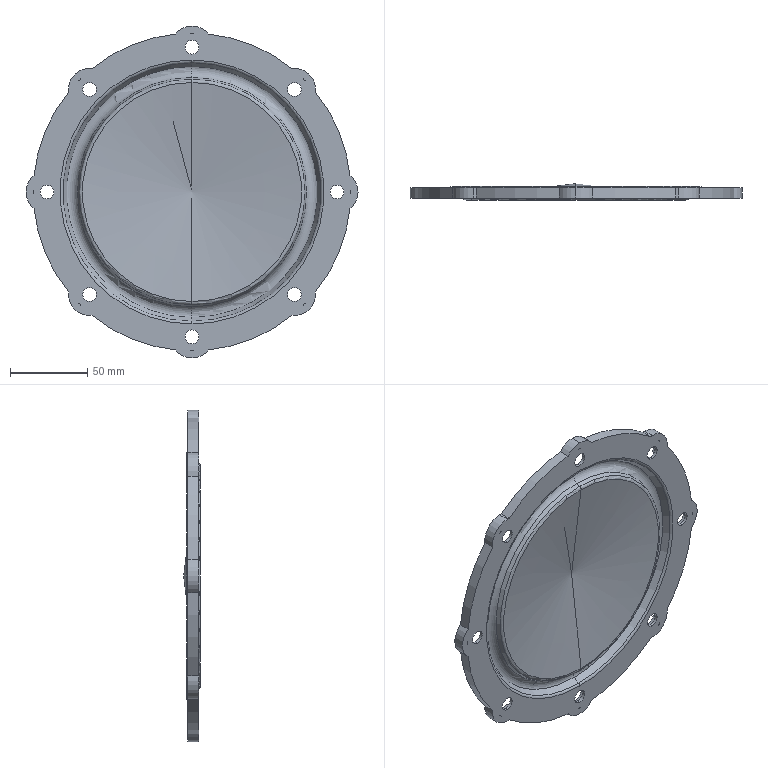Part | SolidWorks | features BaseBody 1 | 1 solid | 86 faces | box 215.352 x 10.74 x 215.352 mm | volume 96271 mm3 | cylinder 63 | cone 12 | torus 8 | plane 3 | commonest cylinder face diameters 206 x17 9 x16 18.083 x11 27.352 x11 190 x8